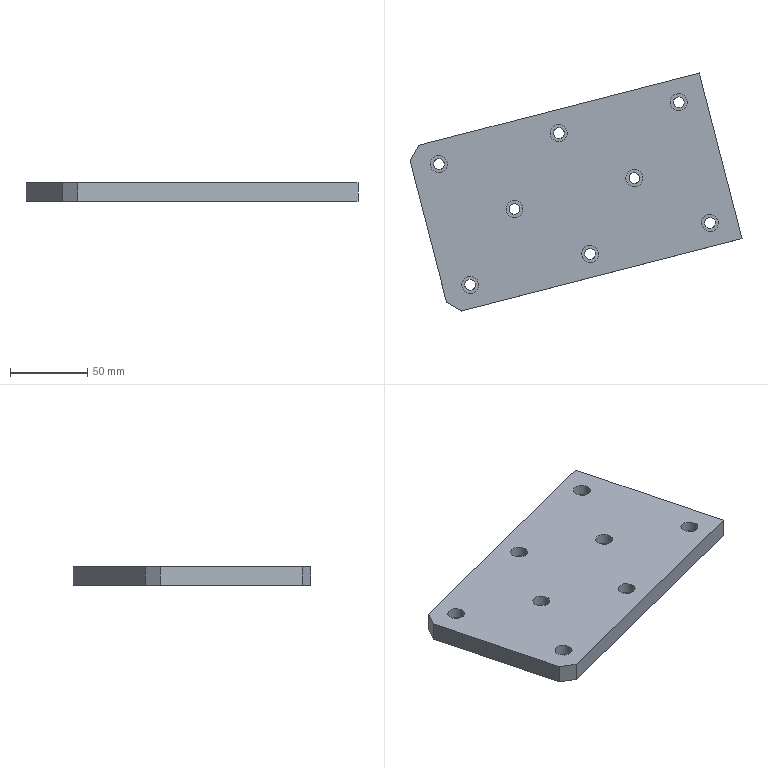Part | STEP file | 车灯-后视镜_id710_x_t | 1 solid | 32 faces | box 214.417 x 153.693 x 12 mm | volume 250941 mm3 | plane 16 | cylinder 16 | commonest cylinder face diameters 7 x8 11 x8
STEP:
#1=CARTESIAN_POINT('',(-441.728,-90.977,-35.286));
#2=VERTEX_POINT('',#1);
#3=CARTESIAN_POINT('',(-465.324,0.5297,-35.286));
#4=VERTEX_POINT('',#3);
#5=CARTESIAN_POINT('',(-453.468,-45.449,-35.286));
#6=DIRECTION('',(-0.2497,0.9683,0.));
#7=VECTOR('',#6,1.);
#8=LINE('',#5,#7);
#9=EDGE_CURVE('',#2,#4,#8,.T.);
#10=ORIENTED_EDGE('',*,*,#9,.T.);
#11=CARTESIAN_POINT('',(-465.324,0.5297,-47.286));
#12=VERTEX_POINT('',#11);
#13=CARTESIAN_POINT('',(-465.324,0.5297,-47.286));
#14=DIRECTION('',(0.,0.,-1.));
#15=VECTOR('',#14,1.);
#16=LINE('',#13,#15);
#17=EDGE_CURVE('',#4,#12,#16,.T.);
#18=ORIENTED_EDGE('',*,*,#17,.T.);
#19=CARTESIAN_POINT('',(-441.728,-90.977,-47.286));
#20=VERTEX_POINT('',#19);
#21=CARTESIAN_POINT('',(-453.468,-45.449,-47.286));
#22=DIRECTION('',(-0.2497,0.9683,0.));
#23=VECTOR('',#22,1.);
#24=LINE('',#21,#23);
#25=EDGE_CURVE('',#20,#12,#24,.T.);
#26=ORIENTED_EDGE('',*,*,#25,.F.);
#27=CARTESIAN_POINT('',(-441.728,-90.977,-100.5));
#28=DIRECTION('',(0.,0.,1.));
#29=VECTOR('',#28,1.);
#30=LINE('',#27,#29);
#31=EDGE_CURVE('',#20,#2,#30,.T.);
#32=ORIENTED_EDGE('',*,*,#31,.T.);
#33=EDGE_LOOP('',(#10,#18,#26,#32));
#34=FACE_OUTER_BOUND('',#33,.T.);
#35=CARTESIAN_POINT('',(-483.305,70.259,-100.5));
#36=DIRECTION('',(-0.9683,-0.2497,0.));
#37=DIRECTION('',(0.2497,-0.9683,0.));
#38=AXIS2_PLACEMENT_3D('',#35,#36,#37);
#39=PLANE('',#38);
#40=ADVANCED_FACE('',(#34),#39,.T.);
#41=CARTESIAN_POINT('',(-370.039,21.486,-47.286));
#42=VERTEX_POINT('',#41);
#43=CARTESIAN_POINT('',(-369.165,18.097,-47.286));
#44=DIRECTION('',(0.,0.,1.));
#45=DIRECTION('',(-0.2497,0.9683,0.));
#46=AXIS2_PLACEMENT_3D('',#43,#44,#45);
#47=CIRCLE('',#46,3.5);
#48=EDGE_CURVE('',#42,#42,#47,.T.);
#49=ORIENTED_EDGE('',*,*,#48,.T.);
#50=EDGE_LOOP('',(#49));
#51=FACE_BOUND('',#50,.T.);
#52=CARTESIAN_POINT('',(-349.938,-56.464,-47.286));
#53=VERTEX_POINT('',#52);
#54=CARTESIAN_POINT('',(-349.064,-59.853,-47.286));
#55=DIRECTION('',(0.,0.,1.));
#56=DIRECTION('',(-0.2497,0.9683,0.));
#57=AXIS2_PLACEMENT_3D('',#54,#55,#56);
#58=CIRCLE('',#57,3.5);
#59=EDGE_CURVE('',#53,#53,#58,.T.);
#60=ORIENTED_EDGE('',*,*,#59,.T.);
#61=EDGE_LOOP('',(#60));
#62=FACE_BOUND('',#61,.T.);
#63=CARTESIAN_POINT('',(-398.721,-27.477,-47.286));
#64=VERTEX_POINT('',#63);
#65=CARTESIAN_POINT('',(-397.848,-30.866,-47.286));
#66=DIRECTION('',(0.,0.,1.));
#67=DIRECTION('',(-0.2497,0.9683,0.));
#68=AXIS2_PLACEMENT_3D('',#65,#66,#67);
#69=CIRCLE('',#68,3.5);
#70=EDGE_CURVE('',#64,#64,#69,.T.);
#71=ORIENTED_EDGE('',*,*,#70,.T.);
#72=EDGE_LOOP('',(#71));
#73=FACE_BOUND('',#72,.T.);
#74=CARTESIAN_POINT('',(-292.573,41.462,-47.286));
#75=VERTEX_POINT('',#74);
#76=CARTESIAN_POINT('',(-291.699,38.073,-47.286));
#77=DIRECTION('',(0.,0.,1.));
#78=DIRECTION('',(-0.2497,0.9683,0.));
#79=AXIS2_PLACEMENT_3D('',#76,#77,#78);
#80=CIRCLE('',#79,3.5);
#81=EDGE_CURVE('',#75,#75,#80,.T.);
#82=ORIENTED_EDGE('',*,*,#81,.T.);
#83=EDGE_LOOP('',(#82));
#84=FACE_BOUND('',#83,.T.);
#85=CARTESIAN_POINT('',(-321.256,-7.501,-47.286));
#86=VERTEX_POINT('',#85);
#87=CARTESIAN_POINT('',(-320.382,-10.89,-47.286));
#88=DIRECTION('',(0.,0.,1.));
#89=DIRECTION('',(-0.2497,0.9683,0.));
#90=AXIS2_PLACEMENT_3D('',#87,#88,#89);
#91=CIRCLE('',#90,3.5);
#92=EDGE_CURVE('',#86,#86,#91,.T.);
#93=ORIENTED_EDGE('',*,*,#92,.T.);
#94=EDGE_LOOP('',(#93));
#95=FACE_BOUND('',#94,.T.);
#96=CARTESIAN_POINT('',(-427.404,-76.44,-47.286));
#97=VERTEX_POINT('',#96);
#98=CARTESIAN_POINT('',(-426.53,-79.829,-47.286));
#99=DIRECTION('',(0.,0.,1.));
#100=DIRECTION('',(-0.2497,0.9683,0.));
#101=AXIS2_PLACEMENT_3D('',#98,#99,#100);
#102=CIRCLE('',#101,3.5);
#103=EDGE_CURVE('',#97,#97,#102,.T.);
#104=ORIENTED_EDGE('',*,*,#103,.T.);
#105=EDGE_LOOP('',(#104));
#106=FACE_BOUND('',#105,.T.);
#107=CARTESIAN_POINT('',(-272.472,-36.488,-47.286));
#108=VERTEX_POINT('',#107);
#109=CARTESIAN_POINT('',(-271.598,-39.877,-47.286));
#110=DIRECTION('',(0.,0.,1.));
#111=DIRECTION('',(-0.2497,0.9683,0.));
#112=AXIS2_PLACEMENT_3D('',#109,#110,#111);
#113=CIRCLE('',#112,3.5);
#114=EDGE_CURVE('',#108,#108,#113,.T.);
#115=ORIENTED_EDGE('',*,*,#114,.T.);
#116=EDGE_LOOP('',(#115));
#117=FACE_BOUND('',#116,.T.);
#118=CARTESIAN_POINT('',(-447.505,1.51,-47.286));
#119=VERTEX_POINT('',#118);
#120=CARTESIAN_POINT('',(-446.631,-1.879,-47.286));
#121=DIRECTION('',(0.,0.,1.));
#122=DIRECTION('',(-0.2497,0.9683,0.));
#123=AXIS2_PLACEMENT_3D('',#120,#121,#122);
#124=CIRCLE('',#123,3.5);
#125=EDGE_CURVE('',#119,#119,#124,.T.);
#126=ORIENTED_EDGE('',*,*,#125,.T.);
#127=EDGE_LOOP('',(#126));
#128=FACE_BOUND('',#127,.T.);
#129=CARTESIAN_POINT('',(-250.907,-50.032,-47.286));
#130=VERTEX_POINT('',#129);
#131=CARTESIAN_POINT('',(-278.499,56.968,-47.286));
#132=VERTEX_POINT('',#131);
#133=CARTESIAN_POINT('',(-264.645,3.242,-47.286));
#134=DIRECTION('',(-0.2497,0.9683,0.));
#135=VECTOR('',#134,1.);
#136=LINE('',#133,#135);
#137=EDGE_CURVE('',#130,#132,#136,.T.);
#138=ORIENTED_EDGE('',*,*,#137,.F.);
#139=CARTESIAN_POINT('',(-431.984,-96.726,-47.286));
#140=VERTEX_POINT('',#139);
#141=CARTESIAN_POINT('',(-81.451,-6.335,-47.286));
#142=DIRECTION('',(-0.9683,-0.2497,0.));
#143=VECTOR('',#142,1.);
#144=LINE('',#141,#143);
#145=EDGE_CURVE('',#130,#140,#144,.T.);
#146=ORIENTED_EDGE('',*,*,#145,.T.);
#147=CARTESIAN_POINT('',(-245.028,-207.029,-47.286));
#148=DIRECTION('',(-0.8613,0.5081,0.));
#149=VECTOR('',#148,1.);
#150=LINE('',#147,#149);
#151=EDGE_CURVE('',#140,#20,#150,.T.);
#152=ORIENTED_EDGE('',*,*,#151,.T.);
#153=ORIENTED_EDGE('',*,*,#25,.T.);
#154=CARTESIAN_POINT('',(-459.575,10.274,-47.286));
#155=VERTEX_POINT('',#154);
#156=CARTESIAN_POINT('',(-349.44,196.946,-47.286));
#157=DIRECTION('',(0.5081,0.8613,0.));
#158=VECTOR('',#157,1.);
#159=LINE('',#156,#158);
#160=EDGE_CURVE('',#12,#155,#159,.T.);
#161=ORIENTED_EDGE('',*,*,#160,.T.);
#162=CARTESIAN_POINT('',(-109.042,100.665,-47.286));
#163=DIRECTION('',(-0.9683,-0.2497,0.));
#164=VECTOR('',#163,1.);
#165=LINE('',#162,#164);
#166=EDGE_CURVE('',#132,#155,#165,.T.);
#167=ORIENTED_EDGE('',*,*,#166,.F.);
#168=EDGE_LOOP('',(#138,#146,#152,#153,#161,#167));
#169=FACE_BOUND('',#168,.T.);
#170=CARTESIAN_POINT('',(-95.188,46.94,-47.286));
#171=DIRECTION('',(0.,0.,-1.));
#172=DIRECTION('',(0.9683,0.2497,0.));
#173=AXIS2_PLACEMENT_3D('',#170,#171,#172);
#174=PLANE('',#173);
#175=ADVANCED_FACE('',(#51,#62,#73,#84,#95,#106,#117,#128,#169),#174,.T.);
#176=CARTESIAN_POINT('',(-367.792,12.771,-35.286));
#177=VERTEX_POINT('',#176);
#178=CARTESIAN_POINT('',(-369.165,18.097,-35.286));
#179=DIRECTION('',(0.,0.,-1.));
#180=DIRECTION('',(0.2497,-0.9683,0.));
#181=AXIS2_PLACEMENT_3D('',#178,#179,#180);
#182=CIRCLE('',#181,5.5);
#183=EDGE_CURVE('',#177,#177,#182,.T.);
#184=ORIENTED_EDGE('',*,*,#183,.T.);
#185=EDGE_LOOP('',(#184));
#186=FACE_BOUND('',#185,.T.);
#187=CARTESIAN_POINT('',(-347.691,-65.179,-35.286));
#188=VERTEX_POINT('',#187);
#189=CARTESIAN_POINT('',(-349.064,-59.853,-35.286));
#190=DIRECTION('',(0.,0.,-1.));
#191=DIRECTION('',(0.2497,-0.9683,0.));
#192=AXIS2_PLACEMENT_3D('',#189,#190,#191);
#193=CIRCLE('',#192,5.5);
#194=EDGE_CURVE('',#188,#188,#193,.T.);
#195=ORIENTED_EDGE('',*,*,#194,.T.);
#196=EDGE_LOOP('',(#195));
#197=FACE_BOUND('',#196,.T.);
#198=CARTESIAN_POINT('',(-396.474,-36.192,-35.286));
#199=VERTEX_POINT('',#198);
#200=CARTESIAN_POINT('',(-397.848,-30.866,-35.286));
#201=DIRECTION('',(0.,0.,-1.));
#202=DIRECTION('',(0.2497,-0.9683,0.));
#203=AXIS2_PLACEMENT_3D('',#200,#201,#202);
#204=CIRCLE('',#203,5.5);
#205=EDGE_CURVE('',#199,#199,#204,.T.);
#206=ORIENTED_EDGE('',*,*,#205,.T.);
#207=EDGE_LOOP('',(#206));
#208=FACE_BOUND('',#207,.T.);
#209=CARTESIAN_POINT('',(-290.326,32.747,-35.286));
#210=VERTEX_POINT('',#209);
#211=CARTESIAN_POINT('',(-291.699,38.073,-35.286));
#212=DIRECTION('',(0.,0.,-1.));
#213=DIRECTION('',(0.2497,-0.9683,0.));
#214=AXIS2_PLACEMENT_3D('',#211,#212,#213);
#215=CIRCLE('',#214,5.5);
#216=EDGE_CURVE('',#210,#210,#215,.T.);
#217=ORIENTED_EDGE('',*,*,#216,.T.);
#218=EDGE_LOOP('',(#217));
#219=FACE_BOUND('',#218,.T.);
#220=CARTESIAN_POINT('',(-319.008,-16.216,-35.286));
#221=VERTEX_POINT('',#220);
#222=CARTESIAN_POINT('',(-320.382,-10.89,-35.286));
#223=DIRECTION('',(0.,0.,-1.));
#224=DIRECTION('',(0.2497,-0.9683,0.));
#225=AXIS2_PLACEMENT_3D('',#222,#223,#224);
#226=CIRCLE('',#225,5.5);
#227=EDGE_CURVE('',#221,#221,#226,.T.);
#228=ORIENTED_EDGE('',*,*,#227,.T.);
#229=EDGE_LOOP('',(#228));
#230=FACE_BOUND('',#229,.T.);
#231=CARTESIAN_POINT('',(-425.157,-85.155,-35.286));
#232=VERTEX_POINT('',#231);
#233=CARTESIAN_POINT('',(-426.53,-79.829,-35.286));
#234=DIRECTION('',(0.,0.,-1.));
#235=DIRECTION('',(0.2497,-0.9683,0.));
#236=AXIS2_PLACEMENT_3D('',#233,#234,#235);
#237=CIRCLE('',#236,5.5);
#238=EDGE_CURVE('',#232,#232,#237,.T.);
#239=ORIENTED_EDGE('',*,*,#238,.T.);
#240=EDGE_LOOP('',(#239));
#241=FACE_BOUND('',#240,.T.);
#242=CARTESIAN_POINT('',(-270.225,-45.203,-35.286));
#243=VERTEX_POINT('',#242);
#244=CARTESIAN_POINT('',(-271.598,-39.877,-35.286));
#245=DIRECTION('',(0.,0.,-1.));
#246=DIRECTION('',(0.2497,-0.9683,0.));
#247=AXIS2_PLACEMENT_3D('',#244,#245,#246);
#248=CIRCLE('',#247,5.5);
#249=EDGE_CURVE('',#243,#243,#248,.T.);
#250=ORIENTED_EDGE('',*,*,#249,.T.);
#251=EDGE_LOOP('',(#250));
#252=FACE_BOUND('',#251,.T.);
#253=CARTESIAN_POINT('',(-445.257,-7.205,-35.286));
#254=VERTEX_POINT('',#253);
#255=CARTESIAN_POINT('',(-446.631,-1.879,-35.286));
#256=DIRECTION('',(0.,0.,-1.));
#257=DIRECTION('',(0.2497,-0.9683,0.));
#258=AXIS2_PLACEMENT_3D('',#255,#256,#257);
#259=CIRCLE('',#258,5.5);
#260=EDGE_CURVE('',#254,#254,#259,.T.);
#261=ORIENTED_EDGE('',*,*,#260,.T.);
#262=EDGE_LOOP('',(#261));
#263=FACE_BOUND('',#262,.T.);
#264=CARTESIAN_POINT('',(-250.907,-50.032,-35.286));
#265=VERTEX_POINT('',#264);
#266=CARTESIAN_POINT('',(-431.984,-96.726,-35.286));
#267=VERTEX_POINT('',#266);
#268=CARTESIAN_POINT('',(-81.451,-6.335,-35.286));
#269=DIRECTION('',(-0.9683,-0.2497,0.));
#270=VECTOR('',#269,1.);
#271=LINE('',#268,#270);
#272=EDGE_CURVE('',#265,#267,#271,.T.);
#273=ORIENTED_EDGE('',*,*,#272,.F.);
#274=CARTESIAN_POINT('',(-278.499,56.968,-35.286));
#275=VERTEX_POINT('',#274);
#276=CARTESIAN_POINT('',(-264.645,3.242,-35.286));
#277=DIRECTION('',(-0.2497,0.9683,0.));
#278=VECTOR('',#277,1.);
#279=LINE('',#276,#278);
#280=EDGE_CURVE('',#265,#275,#279,.T.);
#281=ORIENTED_EDGE('',*,*,#280,.T.);
#282=CARTESIAN_POINT('',(-459.575,10.274,-35.286));
#283=VERTEX_POINT('',#282);
#284=CARTESIAN_POINT('',(-109.042,100.665,-35.286));
#285=DIRECTION('',(-0.9683,-0.2497,0.));
#286=VECTOR('',#285,1.);
#287=LINE('',#284,#286);
#288=EDGE_CURVE('',#275,#283,#287,.T.);
#289=ORIENTED_EDGE('',*,*,#288,.T.);
#290=CARTESIAN_POINT('',(-465.324,0.5297,-35.286));
#291=DIRECTION('',(-0.5081,-0.8613,0.));
#292=VECTOR('',#291,1.);
#293=LINE('',#290,#292);
#294=EDGE_CURVE('',#283,#4,#293,.T.);
#295=ORIENTED_EDGE('',*,*,#294,.T.);
#296=ORIENTED_EDGE('',*,*,#9,.F.);
#297=CARTESIAN_POINT('',(-431.984,-96.726,-35.286));
#298=DIRECTION('',(0.8613,-0.5081,0.));
#299=VECTOR('',#298,1.);
#300=LINE('',#297,#299);
#301=EDGE_CURVE('',#2,#267,#300,.T.);
#302=ORIENTED_EDGE('',*,*,#301,.T.);
#303=EDGE_LOOP('',(#273,#281,#289,#295,#296,#302));
#304=FACE_BOUND('',#303,.T.);
#305=CARTESIAN_POINT('',(-95.188,46.94,-35.286));
#306=DIRECTION('',(0.,0.,-1.));
#307=DIRECTION('',(0.9683,0.2497,0.));
#308=AXIS2_PLACEMENT_3D('',#305,#306,#307);
#309=PLANE('',#308);
#310=ADVANCED_FACE('',(#186,#197,#208,#219,#230,#241,#252,#263,#304),#309,.F.);
#311=CARTESIAN_POINT('',(-250.907,-50.032,-35.286));
#312=DIRECTION('',(0.,0.,-1.));
#313=VECTOR('',#312,1.);
#314=LINE('',#311,#313);
#315=EDGE_CURVE('',#265,#130,#314,.T.);
#316=ORIENTED_EDGE('',*,*,#315,.F.);
#317=ORIENTED_EDGE('',*,*,#272,.T.);
#318=CARTESIAN_POINT('',(-431.984,-96.726,-35.286));
#319=DIRECTION('',(0.,0.,-1.));
#320=VECTOR('',#319,1.);
#321=LINE('',#318,#320);
#322=EDGE_CURVE('',#267,#140,#321,.T.);
#323=ORIENTED_EDGE('',*,*,#322,.T.);
#324=ORIENTED_EDGE('',*,*,#145,.F.);
#325=EDGE_LOOP('',(#316,#317,#323,#324));
#326=FACE_OUTER_BOUND('',#325,.T.);
#327=CARTESIAN_POINT('',(-81.451,-6.335,-35.286));
#328=DIRECTION('',(0.2497,-0.9683,0.));
#329=DIRECTION('',(0.9683,0.2497,0.));
#330=AXIS2_PLACEMENT_3D('',#327,#328,#329);
#331=PLANE('',#330);
#332=ADVANCED_FACE('',(#326),#331,.T.);
#333=ORIENTED_EDGE('',*,*,#288,.F.);
#334=CARTESIAN_POINT('',(-278.499,56.968,-35.286));
#335=DIRECTION('',(0.,0.,-1.));
#336=VECTOR('',#335,1.);
#337=LINE('',#334,#336);
#338=EDGE_CURVE('',#275,#132,#337,.T.);
#339=ORIENTED_EDGE('',*,*,#338,.T.);
#340=ORIENTED_EDGE('',*,*,#166,.T.);
#341=CARTESIAN_POINT('',(-459.575,10.274,-35.286));
#342=DIRECTION('',(0.,0.,1.));
#343=VECTOR('',#342,1.);
#344=LINE('',#341,#343);
#345=EDGE_CURVE('',#155,#283,#344,.T.);
#346=ORIENTED_EDGE('',*,*,#345,.T.);
#347=EDGE_LOOP('',(#333,#339,#340,#346));
#348=FACE_OUTER_BOUND('',#347,.T.);
#349=CARTESIAN_POINT('',(-109.042,100.665,-35.286));
#350=DIRECTION('',(0.2497,-0.9683,0.));
#351=DIRECTION('',(0.9683,0.2497,0.));
#352=AXIS2_PLACEMENT_3D('',#349,#350,#351);
#353=PLANE('',#352);
#354=ADVANCED_FACE('',(#348),#353,.F.);
#355=ORIENTED_EDGE('',*,*,#294,.F.);
#356=ORIENTED_EDGE('',*,*,#345,.F.);
#357=ORIENTED_EDGE('',*,*,#160,.F.);
#358=ORIENTED_EDGE('',*,*,#17,.F.);
#359=EDGE_LOOP('',(#355,#356,#357,#358));
#360=FACE_OUTER_BOUND('',#359,.T.);
#361=CARTESIAN_POINT('',(-465.324,0.5297,-100.5));
#362=DIRECTION('',(-0.8613,0.5081,0.));
#363=DIRECTION('',(-0.5081,-0.8613,0.));
#364=AXIS2_PLACEMENT_3D('',#361,#362,#363);
#365=PLANE('',#364);
#366=ADVANCED_FACE('',(#360),#365,.T.);
#367=ORIENTED_EDGE('',*,*,#301,.F.);
#368=ORIENTED_EDGE('',*,*,#31,.F.);
#369=ORIENTED_EDGE('',*,*,#151,.F.);
#370=ORIENTED_EDGE('',*,*,#322,.F.);
#371=EDGE_LOOP('',(#367,#368,#369,#370));
#372=FACE_OUTER_BOUND('',#371,.T.);
#373=CARTESIAN_POINT('',(-431.984,-96.726,-35.286));
#374=DIRECTION('',(0.5081,0.8613,0.));
#375=DIRECTION('',(-0.8613,0.5081,0.));
#376=AXIS2_PLACEMENT_3D('',#373,#374,#375);
#377=PLANE('',#376);
#378=ADVANCED_FACE('',(#372),#377,.F.);
#379=ORIENTED_EDGE('',*,*,#315,.T.);
#380=ORIENTED_EDGE('',*,*,#137,.T.);
#381=ORIENTED_EDGE('',*,*,#338,.F.);
#382=ORIENTED_EDGE('',*,*,#280,.F.);
#383=EDGE_LOOP('',(#379,#380,#381,#382));
#384=FACE_OUTER_BOUND('',#383,.T.);
#385=CARTESIAN_POINT('',(-250.907,-50.032,-47.286));
#386=DIRECTION('',(-0.9683,-0.2497,0.));
#387=DIRECTION('',(0.2497,-0.9683,0.));
#388=AXIS2_PLACEMENT_3D('',#385,#386,#387);
#389=PLANE('',#388);
#390=ADVANCED_FACE('',(#384),#389,.F.);
#391=CARTESIAN_POINT('',(-450.131,-1.879,-42.286));
#392=VERTEX_POINT('',#391);
#393=CARTESIAN_POINT('',(-446.631,-1.879,-42.286));
#394=DIRECTION('',(0.,0.,1.));
#395=DIRECTION('',(-1.,0.,0.));
#396=AXIS2_PLACEMENT_3D('',#393,#394,#395);
#397=CIRCLE('',#396,3.5);
#398=EDGE_CURVE('',#392,#392,#397,.T.);
#399=ORIENTED_EDGE('',*,*,#398,.T.);
#400=EDGE_LOOP('',(#399));
#401=FACE_BOUND('',#400,.T.);
#402=ORIENTED_EDGE('',*,*,#125,.F.);
#403=EDGE_LOOP('',(#402));
#404=FACE_BOUND('',#403,.T.);
#405=CARTESIAN_POINT('',(-446.631,-1.879,-47.286));
#406=DIRECTION('',(0.,0.,1.));
#407=DIRECTION('',(-0.2497,0.9683,0.));
#408=AXIS2_PLACEMENT_3D('',#405,#406,#407);
#409=CYLINDRICAL_SURFACE('',#408,3.5);
#410=ADVANCED_FACE('',(#401,#404),#409,.F.);
#411=ORIENTED_EDGE('',*,*,#398,.F.);
#412=EDGE_LOOP('',(#411));
#413=FACE_BOUND('',#412,.T.);
#414=CARTESIAN_POINT('',(-448.004,3.447,-42.286));
#415=VERTEX_POINT('',#414);
#416=CARTESIAN_POINT('',(-446.631,-1.879,-42.286));
#417=DIRECTION('',(0.,0.,1.));
#418=DIRECTION('',(-0.2497,0.9683,0.));
#419=AXIS2_PLACEMENT_3D('',#416,#417,#418);
#420=CIRCLE('',#419,5.5);
#421=EDGE_CURVE('',#415,#415,#420,.T.);
#422=ORIENTED_EDGE('',*,*,#421,.T.);
#423=EDGE_LOOP('',(#422));
#424=FACE_BOUND('',#423,.T.);
#425=CARTESIAN_POINT('',(-446.631,-1.879,-42.286));
#426=DIRECTION('',(0.,0.,-1.));
#427=DIRECTION('',(0.2497,-0.9683,0.));
#428=AXIS2_PLACEMENT_3D('',#425,#426,#427);
#429=PLANE('',#428);
#430=ADVANCED_FACE('',(#413,#424),#429,.F.);
#431=ORIENTED_EDGE('',*,*,#421,.F.);
#432=EDGE_LOOP('',(#431));
#433=FACE_BOUND('',#432,.T.);
#434=ORIENTED_EDGE('',*,*,#260,.F.);
#435=EDGE_LOOP('',(#434));
#436=FACE_BOUND('',#435,.T.);
#437=CARTESIAN_POINT('',(-446.631,-1.879,-35.286));
#438=DIRECTION('',(0.,0.,-1.));
#439=DIRECTION('',(0.2497,-0.9683,0.));
#440=AXIS2_PLACEMENT_3D('',#437,#438,#439);
#441=CYLINDRICAL_SURFACE('',#440,5.5);
#442=ADVANCED_FACE('',(#433,#436),#441,.F.);
#443=CARTESIAN_POINT('',(-275.098,-39.877,-42.286));
#444=VERTEX_POINT('',#443);
#445=CARTESIAN_POINT('',(-271.598,-39.877,-42.286));
#446=DIRECTION('',(0.,0.,1.));
#447=DIRECTION('',(-1.,0.,0.));
#448=AXIS2_PLACEMENT_3D('',#445,#446,#447);
#449=CIRCLE('',#448,3.5);
#450=EDGE_CURVE('',#444,#444,#449,.T.);
#451=ORIENTED_EDGE('',*,*,#450,.T.);
#452=EDGE_LOOP('',(#451));
#453=FACE_BOUND('',#452,.T.);
#454=ORIENTED_EDGE('',*,*,#114,.F.);
#455=EDGE_LOOP('',(#454));
#456=FACE_BOUND('',#455,.T.);
#457=CARTESIAN_POINT('',(-271.598,-39.877,-47.286));
#458=DIRECTION('',(0.,0.,1.));
#459=DIRECTION('',(-0.2497,0.9683,0.));
#460=AXIS2_PLACEMENT_3D('',#457,#458,#459);
#461=CYLINDRICAL_SURFACE('',#460,3.5);
#462=ADVANCED_FACE('',(#453,#456),#461,.F.);
#463=ORIENTED_EDGE('',*,*,#450,.F.);
#464=EDGE_LOOP('',(#463));
#465=FACE_BOUND('',#464,.T.);
#466=CARTESIAN_POINT('',(-272.972,-34.551,-42.286));
#467=VERTEX_POINT('',#466);
#468=CARTESIAN_POINT('',(-271.598,-39.877,-42.286));
#469=DIRECTION('',(0.,0.,1.));
#470=DIRECTION('',(-0.2497,0.9683,0.));
#471=AXIS2_PLACEMENT_3D('',#468,#469,#470);
#472=CIRCLE('',#471,5.5);
#473=EDGE_CURVE('',#467,#467,#472,.T.);
#474=ORIENTED_EDGE('',*,*,#473,.T.);
#475=EDGE_LOOP('',(#474));
#476=FACE_BOUND('',#475,.T.);
#477=CARTESIAN_POINT('',(-271.598,-39.877,-42.286));
#478=DIRECTION('',(0.,0.,-1.));
#479=DIRECTION('',(0.2497,-0.9683,0.));
#480=AXIS2_PLACEMENT_3D('',#477,#478,#479);
#481=PLANE('',#480);
#482=ADVANCED_FACE('',(#465,#476),#481,.F.);
#483=ORIENTED_EDGE('',*,*,#473,.F.);
#484=EDGE_LOOP('',(#483));
#485=FACE_BOUND('',#484,.T.);
#486=ORIENTED_EDGE('',*,*,#249,.F.);
#487=EDGE_LOOP('',(#486));
#488=FACE_BOUND('',#487,.T.);
#489=CARTESIAN_POINT('',(-271.598,-39.877,-35.286));
#490=DIRECTION('',(0.,0.,-1.));
#491=DIRECTION('',(0.2497,-0.9683,0.));
#492=AXIS2_PLACEMENT_3D('',#489,#490,#491);
#493=CYLINDRICAL_SURFACE('',#492,5.5);
#494=ADVANCED_FACE('',(#485,#488),#493,.F.);
#495=CARTESIAN_POINT('',(-430.03,-79.829,-42.286));
#496=VERTEX_POINT('',#495);
#497=CARTESIAN_POINT('',(-426.53,-79.829,-42.286));
#498=DIRECTION('',(0.,0.,1.));
#499=DIRECTION('',(-1.,0.,0.));
#500=AXIS2_PLACEMENT_3D('',#497,#498,#499);
#501=CIRCLE('',#500,3.5);
#502=EDGE_CURVE('',#496,#496,#501,.T.);
#503=ORIENTED_EDGE('',*,*,#502,.T.);
#504=EDGE_LOOP('',(#503));
#505=FACE_BOUND('',#504,.T.);
#506=ORIENTED_EDGE('',*,*,#103,.F.);
#507=EDGE_LOOP('',(#506));
#508=FACE_BOUND('',#507,.T.);
#509=CARTESIAN_POINT('',(-426.53,-79.829,-47.286));
#510=DIRECTION('',(0.,0.,1.));
#511=DIRECTION('',(-0.2497,0.9683,0.));
#512=AXIS2_PLACEMENT_3D('',#509,#510,#511);
#513=CYLINDRICAL_SURFACE('',#512,3.5);
#514=ADVANCED_FACE('',(#505,#508),#513,.F.);
#515=ORIENTED_EDGE('',*,*,#502,.F.);
#516=EDGE_LOOP('',(#515));
#517=FACE_BOUND('',#516,.T.);
#518=CARTESIAN_POINT('',(-427.903,-74.503,-42.286));
#519=VERTEX_POINT('',#518);
#520=CARTESIAN_POINT('',(-426.53,-79.829,-42.286));
#521=DIRECTION('',(0.,0.,1.));
#522=DIRECTION('',(-0.2497,0.9683,0.));
#523=AXIS2_PLACEMENT_3D('',#520,#521,#522);
#524=CIRCLE('',#523,5.5);
#525=EDGE_CURVE('',#519,#519,#524,.T.);
#526=ORIENTED_EDGE('',*,*,#525,.T.);
#527=EDGE_LOOP('',(#526));
#528=FACE_BOUND('',#527,.T.);
#529=CARTESIAN_POINT('',(-426.53,-79.829,-42.286));
#530=DIRECTION('',(0.,0.,-1.));
#531=DIRECTION('',(0.2497,-0.9683,0.));
#532=AXIS2_PLACEMENT_3D('',#529,#530,#531);
#533=PLANE('',#532);
#534=ADVANCED_FACE('',(#517,#528),#533,.F.);
#535=ORIENTED_EDGE('',*,*,#525,.F.);
#536=EDGE_LOOP('',(#535));
#537=FACE_BOUND('',#536,.T.);
#538=ORIENTED_EDGE('',*,*,#238,.F.);
#539=EDGE_LOOP('',(#538));
#540=FACE_BOUND('',#539,.T.);
#541=CARTESIAN_POINT('',(-426.53,-79.829,-35.286));
#542=DIRECTION('',(0.,0.,-1.));
#543=DIRECTION('',(0.2497,-0.9683,0.));
#544=AXIS2_PLACEMENT_3D('',#541,#542,#543);
#545=CYLINDRICAL_SURFACE('',#544,5.5);
#546=ADVANCED_FACE('',(#537,#540),#545,.F.);
#547=CARTESIAN_POINT('',(-323.882,-10.89,-42.286));
#548=VERTEX_POINT('',#547);
#549=CARTESIAN_POINT('',(-320.382,-10.89,-42.286));
#550=DIRECTION('',(0.,0.,1.));
#551=DIRECTION('',(-1.,0.,0.));
#552=AXIS2_PLACEMENT_3D('',#549,#550,#551);
#553=CIRCLE('',#552,3.5);
#554=EDGE_CURVE('',#548,#548,#553,.T.);
#555=ORIENTED_EDGE('',*,*,#554,.T.);
#556=EDGE_LOOP('',(#555));
#557=FACE_BOUND('',#556,.T.);
#558=ORIENTED_EDGE('',*,*,#92,.F.);
#559=EDGE_LOOP('',(#558));
#560=FACE_BOUND('',#559,.T.);
#561=CARTESIAN_POINT('',(-320.382,-10.89,-47.286));
#562=DIRECTION('',(0.,0.,1.));
#563=DIRECTION('',(-0.2497,0.9683,0.));
#564=AXIS2_PLACEMENT_3D('',#561,#562,#563);
#565=CYLINDRICAL_SURFACE('',#564,3.5);
#566=ADVANCED_FACE('',(#557,#560),#565,.F.);
#567=ORIENTED_EDGE('',*,*,#554,.F.);
#568=EDGE_LOOP('',(#567));
#569=FACE_BOUND('',#568,.T.);
#570=CARTESIAN_POINT('',(-321.755,-5.564,-42.286));
#571=VERTEX_POINT('',#570);
#572=CARTESIAN_POINT('',(-320.382,-10.89,-42.286));
#573=DIRECTION('',(0.,0.,1.));
#574=DIRECTION('',(-0.2497,0.9683,0.));
#575=AXIS2_PLACEMENT_3D('',#572,#573,#574);
#576=CIRCLE('',#575,5.5);
#577=EDGE_CURVE('',#571,#571,#576,.T.);
#578=ORIENTED_EDGE('',*,*,#577,.T.);
#579=EDGE_LOOP('',(#578));
#580=FACE_BOUND('',#579,.T.);
#581=CARTESIAN_POINT('',(-320.382,-10.89,-42.286));
#582=DIRECTION('',(0.,0.,-1.));
#583=DIRECTION('',(0.2497,-0.9683,0.));
#584=AXIS2_PLACEMENT_3D('',#581,#582,#583);
#585=PLANE('',#584);
#586=ADVANCED_FACE('',(#569,#580),#585,.F.);
#587=ORIENTED_EDGE('',*,*,#577,.F.);
#588=EDGE_LOOP('',(#587));
#589=FACE_BOUND('',#588,.T.);
#590=ORIENTED_EDGE('',*,*,#227,.F.);
#591=EDGE_LOOP('',(#590));
#592=FACE_BOUND('',#591,.T.);
#593=CARTESIAN_POINT('',(-320.382,-10.89,-35.286));
#594=DIRECTION('',(0.,0.,-1.));
#595=DIRECTION('',(0.2497,-0.9683,0.));
#596=AXIS2_PLACEMENT_3D('',#593,#594,#595);
#597=CYLINDRICAL_SURFACE('',#596,5.5);
#598=ADVANCED_FACE('',(#589,#592),#597,.F.);
#599=CARTESIAN_POINT('',(-295.199,38.073,-42.286));
#600=VERTEX_POINT('',#599);
#601=CARTESIAN_POINT('',(-291.699,38.073,-42.286));
#602=DIRECTION('',(0.,0.,1.));
#603=DIRECTION('',(-1.,0.,0.));
#604=AXIS2_PLACEMENT_3D('',#601,#602,#603);
#605=CIRCLE('',#604,3.5);
#606=EDGE_CURVE('',#600,#600,#605,.T.);
#607=ORIENTED_EDGE('',*,*,#606,.T.);
#608=EDGE_LOOP('',(#607));
#609=FACE_BOUND('',#608,.T.);
#610=ORIENTED_EDGE('',*,*,#81,.F.);
#611=EDGE_LOOP('',(#610));
#612=FACE_BOUND('',#611,.T.);
#613=CARTESIAN_POINT('',(-291.699,38.073,-47.286));
#614=DIRECTION('',(0.,0.,1.));
#615=DIRECTION('',(-0.2497,0.9683,0.));
#616=AXIS2_PLACEMENT_3D('',#613,#614,#615);
#617=CYLINDRICAL_SURFACE('',#616,3.5);
#618=ADVANCED_FACE('',(#609,#612),#617,.F.);
#619=ORIENTED_EDGE('',*,*,#606,.F.);
#620=EDGE_LOOP('',(#619));
#621=FACE_BOUND('',#620,.T.);
#622=CARTESIAN_POINT('',(-293.072,43.399,-42.286));
#623=VERTEX_POINT('',#622);
#624=CARTESIAN_POINT('',(-291.699,38.073,-42.286));
#625=DIRECTION('',(0.,0.,1.));
#626=DIRECTION('',(-0.2497,0.9683,0.));
#627=AXIS2_PLACEMENT_3D('',#624,#625,#626);
#628=CIRCLE('',#627,5.5);
#629=EDGE_CURVE('',#623,#623,#628,.T.);
#630=ORIENTED_EDGE('',*,*,#629,.T.);
#631=EDGE_LOOP('',(#630));
#632=FACE_BOUND('',#631,.T.);
#633=CARTESIAN_POINT('',(-291.699,38.073,-42.286));
#634=DIRECTION('',(0.,0.,-1.));
#635=DIRECTION('',(0.2497,-0.9683,0.));
#636=AXIS2_PLACEMENT_3D('',#633,#634,#635);
#637=PLANE('',#636);
#638=ADVANCED_FACE('',(#621,#632),#637,.F.);
#639=ORIENTED_EDGE('',*,*,#629,.F.);
#640=EDGE_LOOP('',(#639));
#641=FACE_BOUND('',#640,.T.);
#642=ORIENTED_EDGE('',*,*,#216,.F.);
#643=EDGE_LOOP('',(#642));
#644=FACE_BOUND('',#643,.T.);
#645=CARTESIAN_POINT('',(-291.699,38.073,-35.286));
#646=DIRECTION('',(0.,0.,-1.));
#647=DIRECTION('',(0.2497,-0.9683,0.));
#648=AXIS2_PLACEMENT_3D('',#645,#646,#647);
#649=CYLINDRICAL_SURFACE('',#648,5.5);
#650=ADVANCED_FACE('',(#641,#644),#649,.F.);
#651=CARTESIAN_POINT('',(-401.348,-30.866,-42.286));
#652=VERTEX_POINT('',#651);
#653=CARTESIAN_POINT('',(-397.848,-30.866,-42.286));
#654=DIRECTION('',(0.,0.,1.));
#655=DIRECTION('',(-1.,0.,0.));
#656=AXIS2_PLACEMENT_3D('',#653,#654,#655);
#657=CIRCLE('',#656,3.5);
#658=EDGE_CURVE('',#652,#652,#657,.T.);
#659=ORIENTED_EDGE('',*,*,#658,.T.);
#660=EDGE_LOOP('',(#659));
#661=FACE_BOUND('',#660,.T.);
#662=ORIENTED_EDGE('',*,*,#70,.F.);
#663=EDGE_LOOP('',(#662));
#664=FACE_BOUND('',#663,.T.);
#665=CARTESIAN_POINT('',(-397.848,-30.866,-47.286));
#666=DIRECTION('',(0.,0.,1.));
#667=DIRECTION('',(-0.2497,0.9683,0.));
#668=AXIS2_PLACEMENT_3D('',#665,#666,#667);
#669=CYLINDRICAL_SURFACE('',#668,3.5);
#670=ADVANCED_FACE('',(#661,#664),#669,.F.);
#671=ORIENTED_EDGE('',*,*,#658,.F.);
#672=EDGE_LOOP('',(#671));
#673=FACE_BOUND('',#672,.T.);
#674=CARTESIAN_POINT('',(-399.221,-25.54,-42.286));
#675=VERTEX_POINT('',#674);
#676=CARTESIAN_POINT('',(-397.848,-30.866,-42.286));
#677=DIRECTION('',(0.,0.,1.));
#678=DIRECTION('',(-0.2497,0.9683,0.));
#679=AXIS2_PLACEMENT_3D('',#676,#677,#678);
#680=CIRCLE('',#679,5.5);
#681=EDGE_CURVE('',#675,#675,#680,.T.);
#682=ORIENTED_EDGE('',*,*,#681,.T.);
#683=EDGE_LOOP('',(#682));
#684=FACE_BOUND('',#683,.T.);
#685=CARTESIAN_POINT('',(-397.848,-30.866,-42.286));
#686=DIRECTION('',(0.,0.,-1.));
#687=DIRECTION('',(0.2497,-0.9683,0.));
#688=AXIS2_PLACEMENT_3D('',#685,#686,#687);
#689=PLANE('',#688);
#690=ADVANCED_FACE('',(#673,#684),#689,.F.);
#691=ORIENTED_EDGE('',*,*,#681,.F.);
#692=EDGE_LOOP('',(#691));
#693=FACE_BOUND('',#692,.T.);
#694=ORIENTED_EDGE('',*,*,#205,.F.);
#695=EDGE_LOOP('',(#694));
#696=FACE_BOUND('',#695,.T.);
#697=CARTESIAN_POINT('',(-397.848,-30.866,-35.286));
#698=DIRECTION('',(0.,0.,-1.));
#699=DIRECTION('',(0.2497,-0.9683,0.));
#700=AXIS2_PLACEMENT_3D('',#697,#698,#699);
#701=CYLINDRICAL_SURFACE('',#700,5.5);
#702=ADVANCED_FACE('',(#693,#696),#701,.F.);
#703=CARTESIAN_POINT('',(-352.564,-59.853,-42.286));
#704=VERTEX_POINT('',#703);
#705=CARTESIAN_POINT('',(-349.064,-59.853,-42.286));
#706=DIRECTION('',(0.,0.,1.));
#707=DIRECTION('',(-1.,0.,0.));
#708=AXIS2_PLACEMENT_3D('',#705,#706,#707);
#709=CIRCLE('',#708,3.5);
#710=EDGE_CURVE('',#704,#704,#709,.T.);
#711=ORIENTED_EDGE('',*,*,#710,.T.);
#712=EDGE_LOOP('',(#711));
#713=FACE_BOUND('',#712,.T.);
#714=ORIENTED_EDGE('',*,*,#59,.F.);
#715=EDGE_LOOP('',(#714));
#716=FACE_BOUND('',#715,.T.);
#717=CARTESIAN_POINT('',(-349.064,-59.853,-47.286));
#718=DIRECTION('',(0.,0.,1.));
#719=DIRECTION('',(-0.2497,0.9683,0.));
#720=AXIS2_PLACEMENT_3D('',#717,#718,#719);
#721=CYLINDRICAL_SURFACE('',#720,3.5);
#722=ADVANCED_FACE('',(#713,#716),#721,.F.);
#723=ORIENTED_EDGE('',*,*,#710,.F.);
#724=EDGE_LOOP('',(#723));
#725=FACE_BOUND('',#724,.T.);
#726=CARTESIAN_POINT('',(-350.438,-54.527,-42.286));
#727=VERTEX_POINT('',#726);
#728=CARTESIAN_POINT('',(-349.064,-59.853,-42.286));
#729=DIRECTION('',(0.,0.,1.));
#730=DIRECTION('',(-0.2497,0.9683,0.));
#731=AXIS2_PLACEMENT_3D('',#728,#729,#730);
#732=CIRCLE('',#731,5.5);
#733=EDGE_CURVE('',#727,#727,#732,.T.);
#734=ORIENTED_EDGE('',*,*,#733,.T.);
#735=EDGE_LOOP('',(#734));
#736=FACE_BOUND('',#735,.T.);
#737=CARTESIAN_POINT('',(-349.064,-59.853,-42.286));
#738=DIRECTION('',(0.,0.,-1.));
#739=DIRECTION('',(0.2497,-0.9683,0.));
#740=AXIS2_PLACEMENT_3D('',#737,#738,#739);
#741=PLANE('',#740);
#742=ADVANCED_FACE('',(#725,#736),#741,.F.);
#743=ORIENTED_EDGE('',*,*,#733,.F.);
#744=EDGE_LOOP('',(#743));
#745=FACE_BOUND('',#744,.T.);
#746=ORIENTED_EDGE('',*,*,#194,.F.);
#747=EDGE_LOOP('',(#746));
#748=FACE_BOUND('',#747,.T.);
#749=CARTESIAN_POINT('',(-349.064,-59.853,-35.286));
#750=DIRECTION('',(0.,0.,-1.));
#751=DIRECTION('',(0.2497,-0.9683,0.));
#752=AXIS2_PLACEMENT_3D('',#749,#750,#751);
#753=CYLINDRICAL_SURFACE('',#752,5.5);
#754=ADVANCED_FACE('',(#745,#748),#753,.F.);
#755=CARTESIAN_POINT('',(-372.665,18.097,-42.286));
#756=VERTEX_POINT('',#755);
#757=CARTESIAN_POINT('',(-369.165,18.097,-42.286));
#758=DIRECTION('',(0.,0.,1.));
#759=DIRECTION('',(-1.,0.,0.));
#760=AXIS2_PLACEMENT_3D('',#757,#758,#759);
#761=CIRCLE('',#760,3.5);
#762=EDGE_CURVE('',#756,#756,#761,.T.);
#763=ORIENTED_EDGE('',*,*,#762,.T.);
#764=EDGE_LOOP('',(#763));
#765=FACE_BOUND('',#764,.T.);
#766=ORIENTED_EDGE('',*,*,#48,.F.);
#767=EDGE_LOOP('',(#766));
#768=FACE_BOUND('',#767,.T.);
#769=CARTESIAN_POINT('',(-369.165,18.097,-47.286));
#770=DIRECTION('',(0.,0.,1.));
#771=DIRECTION('',(-0.2497,0.9683,0.));
#772=AXIS2_PLACEMENT_3D('',#769,#770,#771);
#773=CYLINDRICAL_SURFACE('',#772,3.5);
#774=ADVANCED_FACE('',(#765,#768),#773,.F.);
#775=ORIENTED_EDGE('',*,*,#762,.F.);
#776=EDGE_LOOP('',(#775));
#777=FACE_BOUND('',#776,.T.);
#778=CARTESIAN_POINT('',(-370.538,23.423,-42.286));
#779=VERTEX_POINT('',#778);
#780=CARTESIAN_POINT('',(-369.165,18.097,-42.286));
#781=DIRECTION('',(0.,0.,1.));
#782=DIRECTION('',(-0.2497,0.9683,0.));
#783=AXIS2_PLACEMENT_3D('',#780,#781,#782);
#784=CIRCLE('',#783,5.5);
#785=EDGE_CURVE('',#779,#779,#784,.T.);
#786=ORIENTED_EDGE('',*,*,#785,.T.);
#787=EDGE_LOOP('',(#786));
#788=FACE_BOUND('',#787,.T.);
#789=CARTESIAN_POINT('',(-369.165,18.097,-42.286));
#790=DIRECTION('',(0.,0.,-1.));
#791=DIRECTION('',(0.2497,-0.9683,0.));
#792=AXIS2_PLACEMENT_3D('',#789,#790,#791);
#793=PLANE('',#792);
#794=ADVANCED_FACE('',(#777,#788),#793,.F.);
#795=ORIENTED_EDGE('',*,*,#785,.F.);
#796=EDGE_LOOP('',(#795));
#797=FACE_BOUND('',#796,.T.);
#798=ORIENTED_EDGE('',*,*,#183,.F.);
#799=EDGE_LOOP('',(#798));
#800=FACE_BOUND('',#799,.T.);
#801=CARTESIAN_POINT('',(-369.165,18.097,-35.286));
#802=DIRECTION('',(0.,0.,-1.));
#803=DIRECTION('',(0.2497,-0.9683,0.));
#804=AXIS2_PLACEMENT_3D('',#801,#802,#803);
#805=CYLINDRICAL_SURFACE('',#804,5.5);
#806=ADVANCED_FACE('',(#797,#800),#805,.F.);
#807=CLOSED_SHELL('',(#40,#175,#310,#332,#354,#366,#378,#390,#410,#430,#442,#462,#482,#494,#514,#534,#546,#566,#586,#598,#618,#638,#650,#670,#690,#702,#722,#742,#754,#774,#794,#806));
#808=MANIFOLD_SOLID_BREP('',#807);
#809=(LENGTH_UNIT()NAMED_UNIT(*)SI_UNIT(.MILLI.,.METRE.));
#810=UNCERTAINTY_MEASURE_WITH_UNIT(LENGTH_MEASURE(0.00002),#809,'','');
#811=(NAMED_UNIT(*)PLANE_ANGLE_UNIT()SI_UNIT($,.RADIAN.));
#812=PLANE_ANGLE_MEASURE_WITH_UNIT(PLANE_ANGLE_MEASURE(0.01745),#811);
#813=DIMENSIONAL_EXPONENTS(0.,0.,0.,0.,0.,0.,0.);
#814=(CONVERSION_BASED_UNIT('DEGREE',#812)NAMED_UNIT(#813)PLANE_ANGLE_UNIT());
#815=(NAMED_UNIT(*)SI_UNIT($,.STERADIAN.)SOLID_ANGLE_UNIT());
#816=(GEOMETRIC_REPRESENTATION_CONTEXT(3)GLOBAL_UNCERTAINTY_ASSIGNED_CONTEXT((#810))GLOBAL_UNIT_ASSIGNED_CONTEXT((#809,#814,#815))REPRESENTATION_CONTEXT('',''));
#817=ADVANCED_BREP_SHAPE_REPRESENTATION('',(#808),#816);